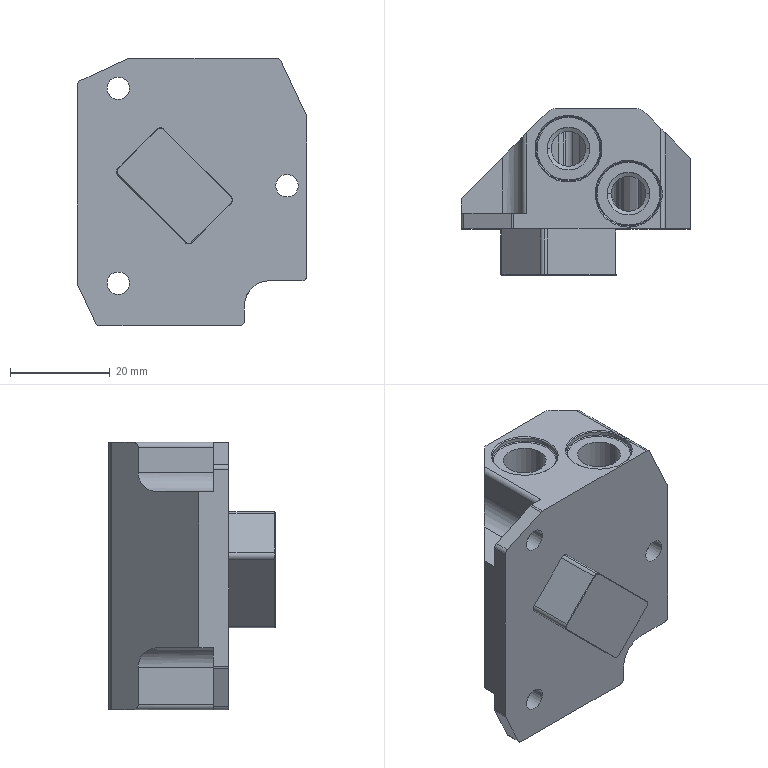NC program | NX | posted with a generic post | part box 46 x 33.25 x 53.5 mm
Lines 2851 to 4234 of 9227:
(动态粗_COPY , TOOL : D5-15-D6-50-3T-ROUGH)
N5694 T03 M6
N5696 G53
N5698 G17 G0 G90 X31.076 Y-9.617 B0. C0. S5500 M3
N5700 G43 Z30.1 H3
N5702 Z-20.3
N5704 G94 G1 X31.051 Y-9.615 Z-20.456 F1500.
N5706 X31.026 Y-9.613 Z-20.518
N5708 X31.001 Y-9.611 Z-20.563
N5710 X30.976 Y-9.609 Z-20.6
N5712 X30.952 Y-9.607 Z-20.631
N5714 X30.927 Y-9.605 Z-20.657
N5716 X30.902 Y-9.603 Z-20.68
N5718 X30.877 Y-9.601 Z-20.7
N5720 X30.852 Y-9.598 Z-20.718
N5722 X30.827 Y-9.596 Z-20.733
N5724 X30.802 Y-9.594 Z-20.747
N5726 X30.777 Y-9.592 Z-20.758
N5728 X30.752 Y-9.59 Z-20.768
N5730 X30.727 Y-9.588 Z-20.777
N5732 X30.702 Y-9.586 Z-20.784
N5734 X30.677 Y-9.584 Z-20.79
N5736 X30.653 Y-9.582 Z-20.794
N5738 X30.628 Y-9.58 Z-20.797
N5740 X30.603 Y-9.578 Z-20.799
N5742 X30.578 Y-9.576 Z-20.8
N5744 X29.881 Y-9.517
N5746 G3 X29.337 Y-9.964 R0.505
N5748 G2 X29.126 Y-11.124 R4.721
N5750 X27.743 Y-15.478 R16.822
N5752 X24.485 Y-22.499 R210.996
N5754 X21.62 Y-24.637 R4.462
N5756 X18.467 Y-25.056 R15.527
N5758 G3 X18.186 Y-25.222 R1.339
N5760 G2 X16.95 Y-25.594 R2.967
N5762 G3 X18.297 Y-25.133 R2.665
N5764 G2 X19.134 Y-24.843 R2.024
N5766 G3 X21.771 Y-24.179 R14.32
N5768 X24.24 Y-21.945 R5.463
N5770 X26.382 Y-17.754 R38.745
N5772 X28.296 Y-13.146 R39.925
N5774 G1 X28.614 Y-12.016
N5776 G3 X29.204 Y-10.81 R3.559
N5778 G2 X28.449 Y-12.237 R3.854
N5780 G3 X27.157 Y-14.833 R19.594
N5782 G2 X24.386 Y-20.629 R79.826
N5784 X20.582 Y-23.809 R6.364
N5786 G3 X19.11 Y-24.321 R69.681
N5788 X18.705 Y-24.807 R2.122
N5790 G1 X18.353 Y-25.088
N5792 G3 X19.059 Y-24.335 R2.54
N5794 G2 X20.592 Y-23.523 R7.508
N5796 G3 X24.162 Y-20.237 R7.733
N5798 X26.636 Y-15.252 R50.491
N5800 G2 X27.833 Y-12.792 R25.129
N5802 G3 X28.551 Y-12.108 R10.707
N5804 G2 X27.648 Y-12.906 R4.578
N5806 G3 X26.327 Y-14.911 R7.951
N5808 G2 X24.13 Y-19.226 R117.584
N5810 X20.404 Y-22.922 R9.092
N5812 G3 X19.4 Y-23.594 R5.764
N5814 X19.102 Y-24.274 R6.577
N5816 G1 X19.035 Y-24.365
N5818 G3 X19.364 Y-23.624 R3.443
N5820 G2 X20.274 Y-22.765 R3.601
N5822 G3 X24.264 Y-18.269 R12.006
N5824 G2 X26.373 Y-14.245 R243.473
N5826 X27.133 Y-13.179 R5.241
N5828 G3 X27.788 Y-12.794 R14.693
N5830 G2 X26.949 Y-13.25 R5.193
N5832 G3 X25.575 Y-14.893 R5.368
N5834 G2 X23.525 Y-18.492 R562.436
N5836 X20.399 Y-21.972 R13.716
N5838 G3 X19.459 Y-22.946 R4.049
N5840 G1 X19.351 Y-23.659
N5842 G2 X19.511 Y-22.778 R3.04
N5844 X20.59 Y-21.491 R5.992
N5846 G3 X24.171 Y-16.732 R18.8
N5848 G2 X25.976 Y-13.884 R19.759
N5850 X26.532 Y-13.366 R2.468
N5852 G1 X27.117 Y-13.162
N5854 G3 X26.179 Y-13.499 R7.877
N5856 X24.693 Y-15.069 R5.396
N5858 G2 X22.527 Y-18.401 R233.076
N5860 X20.094 Y-21.278 R33.455
N5862 G3 X19.445 Y-22.239 R3.013
N5864 G1 X19.435 Y-23.001
N5866 G2 X19.459 Y-22.097 R5.398
N5868 X20.46 Y-20.515 R5.211
N5870 G3 X23.859 Y-15.792 R39.523
N5872 G2 X25.574 Y-13.698 R9.325
N5874 X26.057 Y-13.415 R1.415
N5876 G1 X26.542 Y-13.361
N5878 G3 X25.521 Y-13.563 R2.86
N5880 X23.893 Y-15.066 R5.4
N5882 G1 X21.463 Y-18.418
N5884 G3 X19.635 Y-20.87 R32.6
N5886 X19.435 Y-21.333 R1.332
N5888 G1 Y-22.271
N5890 G2 X19.454 Y-21.126 R24.422
N5892 X20.404 Y-19.386 R5.786
N5894 X23.602 Y-14.996 R166.387
N5896 X25.321 Y-13.478 R5.337
N5898 X25.898 Y-13.433 R9.861
N5900 G3 X25.111 Y-13.481 R7.526
N5902 X23.474 Y-14.611 R3.969
N5904 X20.694 Y-18.143 R37.147
N5906 X19.449 Y-20.142 R10.513
N5908 G1 X19.435 Y-21.274
N5910 G2 X19.454 Y-20.01 R39.949
N5912 X20.44 Y-18.073 R6.448
N5914 X23.284 Y-14.448 R25.188
N5916 X24.707 Y-13.46 R4.137
N5918 G1 X25.306 Y-13.45
N5920 G3 X24.216 Y-13.532 R3.271
N5922 X22.355 Y-14.893 R5.19
N5924 X19.521 Y-18.773 R18.084
N5926 G1 X19.436 Y-19.04
N5928 X19.435 Y-20.165
N5930 X19.452 Y-18.824
N5932 G2 X20.487 Y-16.784 R6.292
N5934 X23.122 Y-13.899 R11.922
N5936 X24.011 Y-13.45 R2.38
N5938 G1 X24.611
N5940 G3 X23.467 Y-13.516 R4.027
N5942 X21.53 Y-14.857 R5.115
N5944 X19.45 Y-17.764 R10.096
N5946 G1 X19.436 Y-18.981
N5948 X19.451 Y-17.645
N5950 G2 X20.552 Y-15.608 R5.519
N5952 X22.87 Y-13.561 R7.086
N5954 X23.202 Y-13.45 R2.139
N5956 G1 X23.802
N5958 G3 X22.657 Y-13.512 R4.284
N5960 X20.539 Y-15.037 R5.056
N5962 X19.447 Y-16.671 R5.979
N5964 G1 X19.436 Y-17.797
N5966 G2 X19.455 Y-16.534 R20.679
N5968 X20.843 Y-14.421 R4.737
N5970 X22.332 Y-13.455 R4.05
N5972 G1 X23.012 Y-13.45
N5974 G3 X21.84 Y-13.511 R4.409
N5976 X19.452 Y-15.697 R4.316
N5978 G1 X19.436 Y-16.702
N5980 G2 X19.457 Y-15.587 R9.901
N5982 X21.553 Y-13.454 R3.485
N5984 G1 X22.153 Y-13.45
N5986 G3 X21.094 Y-13.509 R3.922
N5988 X19.451 Y-14.943 R2.775
N5990 G1 X19.436 Y-15.753
N5992 G2 X19.462 Y-14.824 R4.155
N5994 X20.895 Y-13.452 R2.243
N5996 G1 X21.405 Y-13.45
N5998 G3 X20.386 Y-13.539 R2.784
N6000 X19.516 Y-14.351 R1.427
N6002 X19.436 Y-14.992 R2.942
N6004 G2 X19.926 Y-13.753 R1.462
N6006 X20.573 Y-13.481 R1.202
N6008 X21.173 Y-13.945 R0.505
N6010 G1 X21.192 Y-14.367
N6012 G2 X21.037 Y-14.678 R0.515
N6014 G1 X21.019 Y-14.695 Z-20.799
N6016 X21.001 Y-14.712 Z-20.797
N6018 X20.983 Y-14.73 Z-20.794
N6020 X20.964 Y-14.747 Z-20.79
N6022 X20.946 Y-14.764 Z-20.784
N6024 X20.928 Y-14.781 Z-20.777
N6026 X20.91 Y-14.798 Z-20.768
N6028 X20.892 Y-14.816 Z-20.758
N6030 X20.873 Y-14.833 Z-20.747
N6032 X20.855 Y-14.85 Z-20.733
N6034 X20.837 Y-14.867 Z-20.718
N6036 X20.819 Y-14.884 Z-20.7
N6038 X20.801 Y-14.901 Z-20.68
N6040 X20.783 Y-14.919 Z-20.657
N6042 X20.764 Y-14.936 Z-20.631
N6044 X20.746 Y-14.953 Z-20.6
N6046 X20.728 Y-14.97 Z-20.563
N6048 X20.71 Y-14.987 Z-20.518
N6050 X20.692 Y-15.004 Z-20.456
N6052 X20.674 Y-15.022 Z-20.3
N6054 G0 Z30.1
N6056 X-12.085 Y-26.828
N6058 Z-20.3
N6060 G1 X-12.11 Z-20.456
N6062 X-12.135 Z-20.518
N6064 X-12.16 Z-20.563
N6066 X-12.185 Z-20.6
N6068 X-12.21 Z-20.631
N6070 X-12.235 Z-20.657
N6072 X-12.26 Z-20.68
N6074 X-12.285 Z-20.7
N6076 X-12.31 Z-20.718
N6078 X-12.335 Z-20.733
N6080 X-12.36 Z-20.747
N6082 X-12.385 Z-20.758
N6084 X-12.41 Z-20.768
N6086 X-12.435 Z-20.777
N6088 X-12.46 Z-20.784
N6090 X-12.485 Z-20.79
N6092 X-12.51 Z-20.794
N6094 X-12.535 Z-20.797
N6096 X-12.56 Z-20.799
N6098 X-12.585 Z-20.8
N6100 G2 X-13.047 Y-26.527 R0.506
N6102 G1 X-13.202 Y-26.168
N6104 X-13.373 Y-25.816
N6106 G3 X-13.787 Y-25.6 R0.508
N6108 G2 X-15.607 Y-25.397 R7.506
N6110 X-17.835 Y-25.157 R69.571
N6112 X-21.479 Y-23.892 R17.184
N6114 X-26.417 Y-21.578 R103.757
N6116 X-28.452 Y-18.791 R4.417
N6118 X-28.893 Y-15.038 R16.18
N6120 G1 X-28.954 Y-11.525
N6122 X-29.26 Y-10.651
N6124 G2 X-29.35 Y-9.437 R7.155
N6126 G3 X-28.917 Y-11.57 R4.292
N6128 G2 X-28.642 Y-14.012 R11.018
N6130 G3 X-28.304 Y-17.814 R25.107
N6132 X-25.963 Y-21.251 R5.114
N6134 X-21.906 Y-23.363 R29.004
N6136 X-18.168 Y-24.708 R18.402
N6138 G1 X-15.887 Y-25.08
N6140 G3 X-15.009 Y-25.511 R3.058
N6142 G2 X-16.006 Y-24.976 R2.885
N6144 G3 X-17.82 Y-24.332 R9.627
N6146 G2 X-24.99 Y-21.198 R32.607
N6148 X-27.623 Y-17.462 R5.932
N6150 X-28.125 Y-13.845 R21.529
N6152 G3 X-28.335 Y-12.362 R7.06
N6154 G2 X-28.984 Y-11.428 R6.039
N6156 G3 X-28.335 Y-12.327 R3.58
N6158 G2 X-27.887 Y-13.954 R4.664
N6160 G3 X-27.299 Y-17.276 R24.892
N6162 X-24.464 Y-21.028 R6.502
N6164 X-18.113 Y-23.906 R26.819
N6166 G2 X-16.446 Y-24.518 R11.795
N6168 G1 X-16.174 Y-24.838
N6170 X-15.936 Y-25.021
N6172 G2 X-16.504 Y-24.42 R2.303
N6174 G3 X-18.187 Y-23.466 R5.904
N6176 G2 X-22.785 Y-21.386 R52.481
N6178 X-25.637 Y-19.034 R8.191
N6180 X-27.048 Y-15.506 R9.268
N6182 G3 X-27.651 Y-12.973 R18.748
N6184 X-27.995 Y-12.665 R0.838
N6186 G1 X-28.366 Y-12.293
N6188 G3 X-27.725 Y-12.837 R2.213
N6190 G2 X-27.098 Y-14.225 R3.503
N6192 G3 X-26.135 Y-17.336 R22.654
N6194 X-22.893 Y-20.88 R7.855
N6196 X-18.602 Y-22.962 R33.207
N6198 G2 X-16.774 Y-23.949 R8.305
N6200 X-16.587 Y-24.3 R1.523
N6202 G1 X-16.45 Y-24.479
N6204 G2 X-16.774 Y-23.879 R2.246
N6206 G3 X-18.238 Y-22.732 R4.268
N6208 G2 X-21.662 Y-20.972 R473.58
N6210 X-24.938 Y-18.088 R8.981
N6212 X-26.19 Y-15.326 R12.038
N6214 G3 X-27. Y-13.299 R10.69
N6216 X-27.312 Y-13.093 R0.723
N6218 G1 X-27.757 Y-12.814
N6220 G3 X-27.035 Y-13.222 R7.421
N6222 G2 X-26.21 Y-14.598 R3.981
N6224 G3 X-24.829 Y-17.552 R19.21
N6226 X-21.397 Y-20.704 R9.675
N6228 G1 X-18.113 Y-22.49
N6230 G2 X-16.921 Y-23.437 R4.496
N6232 G1 X-16.863 Y-23.575
N6234 G2 X-16.99 Y-24.042 R0.502
N6236 G1 X-17.379 Y-24.342 Z-20.75
N6238 X-17.775 Y-24.633 Z-20.7
N6240 X-18.116 Y-24.878 F15000.
N6242 G2 X-18.777 Y-24.68 R0.5
N6244 G1 X-18.865 Y-24.527
N6246 X-18.925 Y-24.362
N6248 G2 X-18.055 Y-23.947 R0.5
N6250 G1 X-17.781 Y-24.247 Z-20.741 F1500.
N6252 X-17.498 Y-24.538 Z-20.783
N6254 X-17.349 Y-24.617 Z-20.8
N6256 G3 X-16.732 Y-23.95 R0.5
N6258 G2 X-16.924 Y-23.331 R3.912
N6260 G3 X-18.193 Y-22.05 R3.71
N6262 X-21.234 Y-20.187 R165.735
N6264 G2 X-25.128 Y-15.659 R10.283
N6266 G3 X-26.236 Y-13.621 R13.141
N6268 X-26.553 Y-13.359 R0.755
N6270 G1 X-27.154 Y-13.149
N6272 G2 X-26.305 Y-13.479 R4.099
N6274 X-25.199 Y-14.979 R5.065
N6276 G3 X-23.192 Y-18.028 R15.991
N6278 X-20.093 Y-20.498 R13.845
N6280 G2 X-17.562 Y-22.236 R18.05
N6282 X-16.928 Y-23.058 R2.046
N6284 G1 X-16.869 Y-23.504
N6286 G3 X-17.094 Y-22.518 R2.548
N6288 X-18.645 Y-20.954 R5.492
N6290 G2 X-21.491 Y-18.859 R49.445
N6292 X-24.182 Y-15.62 R13.293
N6294 G3 X-25.592 Y-13.661 R10.79
N6296 X-25.975 Y-13.425 R0.85
N6298 G1 X-26.551 Y-13.36
N6300 G2 X-25.771 Y-13.475 R3.56
N6302 X-24.563 Y-14.634 R3.768
N6304 G3 X-22.429 Y-17.445 R33.621
N6306 X-19.235 Y-20.148 R20.206
N6308 G2 X-17.235 Y-21.954 R9.286
N6310 X-16.936 Y-22.974 R1.272
N6312 G3 X-17.496 Y-21.247 R2.183
N6314 X-19.239 Y-19.599 R12.076
N6316 G2 X-23.501 Y-15.2 R20.861
N6318 G3 X-25.085 Y-13.525 R7.47
N6320 X-25.751 Y-13.45 R1.357
N6322 G1 X-25.937 Y-13.429
N6324 X-25.22 Y-13.452
N6326 G2 X-24.01 Y-14.274 R2.795
N6328 X-21.862 Y-16.738 R121.025
N6330 G3 X-18.752 Y-19.617 R34.105
N6332 G2 X-17.072 Y-21.512 R7.478
N6334 X-16.936 Y-21.884 R1.731
N6336 G1 Y-22.446
N6338 G3 X-16.995 Y-21.391 R3.87
N6340 X-18.224 Y-19.591 R4.969
N6342 G2 X-21.057 Y-16.815 R194.434
N6344 G3 X-23.468 Y-14.185 R85.675
N6346 X-24.45 Y-13.467 R3.465
N6348 G1 X-25.27 Y-13.45
N6350 G2 X-24.35 Y-13.472 R7.141
N6352 X-22.799 Y-14.553 R4.233
N6354 G3 X-18.255 Y-19.159 R172.662
N6356 G2 X-16.946 Y-21.035 R5.661
N6358 G1 X-16.936 Y-21.71
N6360 G3 X-17. Y-20.559 R4.188
N6362 X-18.242 Y-18.615 R5.756
N6364 X-22.362 Y-14.335 R107.426
N6366 X-23.569 Y-13.47 R5.09
N6368 X-24.504 Y-13.45 R10.48
N6370 G2 X-23.47 Y-13.472 R9.077
N6372 X-21.855 Y-14.507 R4.566
N6374 X-17.78 Y-18.755 R46.322
N6376 X-16.941 Y-20.2 R4.92
N6378 G1 X-16.936 Y-20.919
N6380 G3 X-16.992 Y-19.696 R5.168
N6382 X-18.23 Y-17.611 R6.185
N6384 X-21.842 Y-13.955 R25.45
N6386 X-22.703 Y-13.454 R2.671
N6388 G1 X-23.64 Y-13.45
N6390 G2 X-22.524 Y-13.473 R8.444
N6392 X-20.766 Y-14.572 R4.957
N6394 X-17.418 Y-18.291 R19.641
N6396 X-16.936 Y-19.321 R3.21
N6398 G1 Y-20.033
N6400 G3 X-16.984 Y-18.765 R6.188
N6402 X-18.238 Y-16.564 R6.312
N6404 X-21.282 Y-13.665 R13.419
N6406 X-21.775 Y-13.45 R1.294
N6408 G1 X-22.675
N6410 G2 X-21.558 Y-13.47 R11.954
N6412 X-19.785 Y-14.563 R4.796
N6414 X-17.095 Y-17.881 R11.319
N6416 X-16.936 Y-18.338 R2.62
N6418 G1 Y-19.088
N6420 G3 X-16.988 Y-17.753 R6.433
N6422 X-18.307 Y-15.48 R6.168
N6424 X-20.661 Y-13.479 R7.824
N6426 X-21.707 Y-13.45 R5.938
N6428 G2 X-20.595 Y-13.469 R17.143
N6430 X-18.774 Y-14.647 R4.564
N6432 X-16.949 Y-17.249 R7.142
N6434 G1 X-16.936 Y-18.083
N6436 G3 X-16.983 Y-16.772 R6.605
N6438 X-18.644 Y-14.26 R5.568
N6440 X-19.808 Y-13.46 R3.617
N6442 G1 X-20.745 Y-13.45
N6444 G2 X-19.669 Y-13.471 R9.363
N6446 X-17.898 Y-14.744 R4.011
N6448 X-16.939 Y-16.341 R4.52
N6450 G1 X-16.936 Y-17.091
N6452 G3 X-16.987 Y-15.823 R5.741
N6454 X-18.918 Y-13.477 R4.112
N6456 X-19.808 Y-13.45 R4.003
N6458 G2 X-18.844 Y-13.474 R5.75
N6460 X-16.937 Y-15.499 R3.221
N6462 G1 X-16.936 Y-16.149
N6464 G3 X-16.975 Y-15.061 R4.878
N6466 X-18.259 Y-13.472 R2.592
N6468 X-19.013 Y-13.45 R5.62
N6470 G2 X-18.153 Y-13.48 R3.964
N6472 X-16.939 Y-14.792 R2.113
N6474 G1 X-16.936 Y-15.316
N6476 G3 X-17.11 Y-14.14 R2.379
N6478 X-18.188 Y-13.46 R1.281
N6480 G1 X-18.325 Y-13.45
N6482 G2 X-17.304 Y-13.848 R1.499
N6484 X-16.99 Y-14.457 R1.399
N6486 X-17.54 Y-15.05 R0.505
N6488 G1 X-18.164 Y-14.984
N6490 X-18.189 Y-14.981 Z-20.799
N6492 X-18.213 Y-14.979 Z-20.797
N6494 X-18.238 Y-14.976 Z-20.794
N6496 X-18.263 Y-14.973 Z-20.79
N6498 X-18.288 Y-14.971 Z-20.784
N6500 X-18.313 Y-14.968 Z-20.777
N6502 X-18.338 Y-14.965 Z-20.768
N6504 X-18.363 Y-14.963 Z-20.758
N6506 X-18.387 Y-14.96 Z-20.747
N6508 X-18.412 Y-14.957 Z-20.733
N6510 X-18.437 Y-14.955 Z-20.718
N6512 X-18.462 Y-14.952 Z-20.7
N6514 X-18.487 Y-14.949 Z-20.68
N6516 X-18.512 Y-14.947 Z-20.657
N6518 X-18.537 Y-14.944 Z-20.631
N6520 X-18.561 Y-14.942 Z-20.6
N6522 X-18.586 Y-14.939 Z-20.563
N6524 X-18.611 Y-14.936 Z-20.518
N6526 X-18.636 Y-14.934 Z-20.456
N6528 X-18.661 Y-14.931 Z-20.3
N6530 G0 Z30.1
N6532 X-24.518 Y14.833
N6534 Z-6.433
N6536 G1 X-24.519 Y14.808 Z-6.589
N6538 X-24.52 Y14.784 Z-6.651
N6540 X-24.521 Y14.759 Z-6.697
N6542 X-24.522 Y14.734 Z-6.733
N6544 X-24.523 Y14.709 Z-6.764
N6546 X-24.524 Y14.684 Z-6.79
N6548 X-24.525 Y14.659 Z-6.813
N6550 X-24.526 Y14.634 Z-6.833
N6552 X-24.527 Y14.609 Z-6.851
N6554 X-24.528 Y14.584 Z-6.866
N6556 X-24.529 Y14.559 Z-6.88
N6558 X-24.53 Y14.534 Z-6.892
N6560 X-24.531 Y14.509 Z-6.902
N6562 X-24.532 Y14.484 Z-6.91
N6564 X-24.533 Y14.459 Z-6.917
N6566 X-24.534 Y14.434 Z-6.923
N6568 X-24.535 Y14.409 Z-6.928
N6570 X-24.536 Y14.384 Z-6.931
N6572 X-24.537 Y14.359 Z-6.933
N6574 X-24.538 Y14.334
N6576 X-24.567 Y13.635
N6578 G3 X-24.059 Y13.109 R0.505
N6580 X-22.612 Y13.242 R4.347
N6582 X-20.35 Y15.655 R3.586
N6584 G1 Y17.043
N6586 G2 X-20.38 Y15.307 R14.49
N6588 X-22.485 Y13.123 R3.25
N6590 G1 X-23.235 Y13.115
N6592 G3 X-21.88 Y13.269 R3.479
N6594 X-20.362 Y15.398 R2.372
N6596 X-20.975 Y15.947 R0.505
N6598 G1 X-21.581 Y15.81
N6600 X-21.605 Y15.804
N6602 X-21.629 Y15.799 Z-6.931
N6604 X-21.654 Y15.793 Z-6.928
N6606 X-21.678 Y15.788 Z-6.923
N6608 X-21.703 Y15.782 Z-6.917
N6610 X-21.727 Y15.777 Z-6.91
N6612 X-21.751 Y15.771 Z-6.902
N6614 X-21.776 Y15.766 Z-6.892
N6616 X-21.8 Y15.76 Z-6.88
N6618 X-21.825 Y15.755 Z-6.866
N6620 X-21.849 Y15.749 Z-6.851
N6622 X-21.873 Y15.744 Z-6.833
N6624 X-21.898 Y15.738 Z-6.813
N6626 X-21.922 Y15.733 Z-6.79
N6628 X-21.946 Y15.727 Z-6.764
N6630 X-21.971 Y15.722 Z-6.733
N6632 X-21.995 Y15.716 Z-6.697
N6634 X-22.02 Y15.71 Z-6.651
N6636 X-22.044 Y15.705 Z-6.589
N6638 X-22.068 Y15.699 Z-6.433
N6640 G0 Z30.1
N6642 X-24.57 Y14.824
N6644 Z-13.367
N6646 G1 X-24.571 Y14.799 Z-13.523
N6648 X-24.573 Y14.774 Z-13.585
N6650 X-24.574 Y14.749 Z-13.63
N6652 X-24.575 Y14.724 Z-13.667
N6654 X-24.576 Y14.699 Z-13.697
N6656 X-24.577 Y14.674 Z-13.724
N6658 X-24.578 Y14.649 Z-13.747
N6660 X-24.579 Y14.624 Z-13.767
N6662 X-24.58 Y14.599 Z-13.784
N6664 X-24.582 Y14.574 Z-13.8
N6666 X-24.583 Y14.549 Z-13.813
N6668 X-24.584 Y14.524 Z-13.825
N6670 X-24.585 Y14.5 Z-13.835
N6672 X-24.586 Y14.475 Z-13.844
N6674 X-24.587 Y14.45 Z-13.851
N6676 X-24.588 Y14.425 Z-13.857
N6678 X-24.589 Y14.4 Z-13.861
N6680 X-24.59 Y14.375 Z-13.864
N6682 X-24.592 Y14.35 Z-13.866
N6684 X-24.593 Y14.325 Z-13.867
N6686 X-24.624 Y13.628
N6688 G3 X-24.119 Y13.1 R0.505
N6690 X-22.613 Y13.247 R4.23
N6692 X-20.35 Y15.689 R3.585
N6694 G1 Y17.039
N6696 G2 X-20.371 Y15.394 R23.318
N6698 X-22.518 Y13.115 R3.248
N6700 G1 X-23.367 Y13.1
N6702 G3 X-21.88 Y13.269 R3.867
N6704 X-20.35 Y15.606 R2.439
N6706 X-20.803 Y16.108 R0.505
N6708 G1 X-21.581 Y16.188
N6710 X-21.606 Y16.19 Z-13.866
N6712 X-21.631 Y16.193 Z-13.864
N6714 X-21.655 Y16.195 Z-13.861
N6716 X-21.68 Y16.198 Z-13.857
N6718 X-21.705 Y16.201 Z-13.851
N6720 X-21.73 Y16.203 Z-13.844
N6722 X-21.755 Y16.206 Z-13.835
N6724 X-21.78 Y16.208 Z-13.825
N6726 X-21.805 Y16.211 Z-13.813
N6728 X-21.83 Y16.213 Z-13.8
N6730 X-21.854 Y16.216 Z-13.784
N6732 X-21.879 Y16.218 Z-13.767
N6734 X-21.904 Y16.221 Z-13.747
N6736 X-21.929 Y16.224 Z-13.724
N6738 X-21.954 Y16.226 Z-13.697
N6740 X-21.979 Y16.229 Z-13.667
N6742 X-22.004 Y16.231 Z-13.63
N6744 X-22.029 Y16.234 Z-13.585
N6746 X-22.053 Y16.236 Z-13.523
N6748 X-22.078 Y16.239 Z-13.367
N6750 G0 Z30.1
N6752 X-24.53 Y14.832
N6754 Z-20.3
N6756 G1 X-24.532 Y14.807 Z-20.456
N6758 X-24.533 Y14.782 Z-20.518
N6760 X-24.534 Y14.757 Z-20.563
N6762 X-24.535 Y14.732 Z-20.6
N6764 X-24.536 Y14.707 Z-20.631
N6766 X-24.538 Y14.682 Z-20.657
N6768 X-24.539 Y14.657 Z-20.68
N6770 X-24.54 Y14.632 Z-20.7
N6772 X-24.541 Y14.607 Z-20.718
N6774 X-24.543 Y14.582 Z-20.733
N6776 X-24.544 Y14.557 Z-20.747
N6778 X-24.545 Y14.532 Z-20.758
N6780 X-24.546 Y14.507 Z-20.768
N6782 X-24.547 Y14.482 Z-20.777
N6784 X-24.549 Y14.457 Z-20.784
N6786 X-24.55 Y14.432 Z-20.79
N6788 X-24.551 Y14.407 Z-20.794
N6790 X-24.552 Y14.382 Z-20.797
N6792 X-24.554 Y14.358 Z-20.799
N6794 X-24.555 Y14.333 Z-20.8
N6796 X-24.589 Y13.64
N6798 G3 X-24.081 Y13.11 R0.505
N6800 X-22.616 Y13.248 R4.366
N6802 X-20.35 Y15.667 R3.615
N6804 G1 Y17.054
N6806 G2 X-20.376 Y15.358 R16.596
N6808 X-22.535 Y13.119 R3.185
N6810 G1 X-23.322 Y13.115
N6812 G3 X-21.989 Y13.23 R4.057
N6814 X-20.35 Y15.568 R2.404
N6816 X-20.799 Y16.07 R0.505
N6818 G1 X-21.581 Y16.158
N6820 X-21.606 Y16.16 Z-20.799
N6822 X-21.631 Y16.163 Z-20.797
N6824 X-21.655 Y16.166 Z-20.794
N6826 X-21.68 Y16.169 Z-20.79
N6828 X-21.705 Y16.171 Z-20.784
N6830 X-21.73 Y16.174 Z-20.777
N6832 X-21.755 Y16.177 Z-20.768
N6834 X-21.78 Y16.18 Z-20.758
N6836 X-21.804 Y16.183 Z-20.747
N6838 X-21.829 Y16.185 Z-20.733
N6840 X-21.854 Y16.188 Z-20.718
N6842 X-21.879 Y16.191 Z-20.7
N6844 X-21.904 Y16.194 Z-20.68
N6846 X-21.929 Y16.196 Z-20.657
N6848 X-21.954 Y16.199 Z-20.631
N6850 X-21.978 Y16.202 Z-20.6
N6852 X-22.003 Y16.205 Z-20.563
N6854 X-22.028 Y16.208 Z-20.518
N6856 X-22.053 Y16.21 Z-20.456
N6858 X-22.078 Y16.213 Z-20.3
N6860 G0 Z30.1
N6862 X-22.07 Y19.402
N6864 Z-6.433
N6866 G1 X-22.045 Y19.397 Z-6.589
N6868 X-22.021 Y19.393 Z-6.651
N6870 X-21.996 Y19.388 Z-6.697
N6872 X-21.972 Y19.383 Z-6.733
N6874 X-21.947 Y19.378 Z-6.764
N6876 X-21.923 Y19.373 Z-6.79
N6878 X-21.898 Y19.368 Z-6.813
N6880 X-21.874 Y19.363 Z-6.833
N6882 X-21.849 Y19.359 Z-6.851
N6884 X-21.825 Y19.354 Z-6.866
N6886 X-21.8 Y19.349 Z-6.88
N6888 X-21.776 Y19.344 Z-6.892
N6890 X-21.751 Y19.339 Z-6.902
N6892 X-21.727 Y19.334 Z-6.91
N6894 X-21.702 Y19.329 Z-6.917
N6896 X-21.678 Y19.325 Z-6.923
N6898 X-21.653 Y19.32 Z-6.928
N6900 X-21.628 Y19.315 Z-6.931
N6902 X-21.604 Y19.31 Z-6.933
N6904 X-21.579 Y19.305
N6906 X-21.223 Y19.231
N6908 X-20.863 Y19.173
N6910 G3 X-20.359 Y19.683 R0.505
N6912 G2 X-20.008 Y21.245 R3.266
N6914 X-18.427 Y22.479 R2.827
N6916 G1 X-17.749 Y22.575
N6918 X-2.649
N6920 G2 X-0.803 Y21.793 R2.82
N6922 G3 X0.746 Y21.074 R3.932
N6924 X3.114 Y21.564 R4.522
N6926 G2 X4.473 Y22.479 R2.867
N6928 G1 X5.151 Y22.575
N6930 X21.476
N6932 G2 X22.391 Y22.403 R3.105
N6934 G3 X23.017 Y23.074 R0.5
N6936 X22.74 Y23.362 Z-6.892 R0.728
N6938 G1 X22.276 Y23.705 Z-6.833
N6940 X21.899 Y23.988 F15000.
N6942 X21.516 Y24.261
N6944 X21.404 Y24.301
N6946 X21.286 Y24.317
N6948 X9.168
N6950 G3 X5.176 Y24.081 R34.003
N6952 G1 X3.187 Y23.844
N6954 G3 X2.791 Y23.141 R0.5
N6956 G1 X2.846 Y23.019
N6958 X3.251 Y22.124 Z-6.933 F1500.
N6960 G2 X3.187 Y21.634 R0.502
N6962 X2.065 Y21.019 R2.104
N6964 X-0.508 Y21.409 R3.053
N6966 G1 X-0.803 Y21.793
N6968 G3 X0.02 Y20.942 R2.619
N6970 X2.717 Y20.979 R2.924
N6972 G1 X2.856 Y21.154
N6974 G3 X2.806 Y21.669 R0.552
N6976 X2.317 Y21.922 Z-6.875 R0.596
N6978 G1 X1.91 Y21.966 Z-6.833
N6980 X0.497 Y22.119 F15000.
N6982 X-0.003 Y22.168 Z-6.885 F1500.
N6984 G3 X-0.416 Y21.956 Z-6.933 R0.559
N6986 X-0.421 Y21.287 R0.551
N6988 X0.816 Y20.443 R1.68
N6990 X2.564 Y20.639 R2.514
N6992 X2.893 Y21.245 R1.388
N6994 G1 X3.164 Y21.604
N6996 G3 X2.684 Y20.737 R2.228
N6998 G2 X1.628 Y20.256 R1.48
N7000 X-0.18 Y20.788 R2.26
N7002 X-0.373 Y21.204 R5.722
N7004 G3 X0.123 Y20.403 R1.562
N7006 X2.47 Y20.302 R2.112
N7008 X2.624 Y20.555 R1.204
N7010 X2.518 Y21.033 R0.553
N7012 X2.079 Y21.246 Z-6.882 R0.615
N7014 G1 X1.604 Y21.318 Z-6.833
N7016 X0.865 Y21.431 F15000.
N7018 X0.317 Y21.508 Z-6.89 F1500.
N7020 G3 X-0.069 Y21.348 Z-6.933 R0.566
N7022 X-0.19 Y20.752 R0.551
N7024 X0.93 Y19.842 R1.458
N7026 X2.446 Y20.075 R1.763
N7028 X2.635 Y20.612 R0.767
N7030 G1 X2.706 Y20.785
N7032 G3 X2.577 Y20.22 R1.964
N7034 G2 X1.677 Y19.682 R1.129
N7036 X-0.057 Y20.312 R1.826
N7038 G1 X-0.112 Y20.451
N7040 G2 X0.063 Y20.978 R0.552
N7042 X0.588 Y21.099 Z-6.876 R0.601
N7044 G1 X1.007 Y21.046 Z-6.833
N7046 X1.463 Y20.989 F15000.
N7048 X2.197 Y20.891 Z-6.909 F1500.
N7050 X2.308 Y20.844 Z-6.921
N7052 X2.408 Y20.778 Z-6.933
N7054 G2 X2.595 Y20.292 R0.552
N7056 X1.983 Y19.665 R0.849
N7058 X-0.013 Y20.106 R1.823
N7060 X-0.134 Y20.612 R1.134
N7062 G3 X0.005 Y19.978 R1.387
N7064 X2.433 Y19.724 R1.709
N7066 X2.593 Y20.274 R0.907
N7068 G2 X2.438 Y19.683 R1.097
N7070 X0.596 Y19.374 R1.629
N7072 X-0.059 Y20.005 R1.006
N7074 G1 X-0.087 Y20.229
N7076 G3 X0.695 Y19.154 R1.087
N7078 X2.457 Y19.474 R1.575
N7080 X2.55 Y19.934 R0.768
N7082 G2 X2.062 Y19.091 R0.771
N7084 X0.003 Y19.572 R1.621
N7086 X-0.05 Y19.932 R1.053
N7088 G3 X0.483 Y18.956 R0.933
N7090 X2.445 Y19.161 R1.611
N7092 X2.55 Y19.708 R0.807
N7094 G2 X2.044 Y18.782 R0.827
N7096 X0.003 Y19.283 R1.598
N7098 X-0.05 Y19.67 R1.07
N7100 G3 X0.573 Y18.605 R1.
N7102 X2.459 Y18.883 R1.572
N7104 X2.55 Y19.414 R0.858
N7106 G2 X2.389 Y18.739 R0.848
N7108 X-0.009 Y19.016 R1.562
N7110 X-0.05 Y19.38 R1.439
N7112 G3 X0.565 Y18.308 R1.006
N7114 X2.399 Y18.521 R1.585
N7116 X2.55 Y19.091 R1.114
N7118 G2 X2.283 Y18.352 R1.
N7120 X0.009 Y18.69 R1.551
N7122 X-0.05 Y19.089 R2.062
N7124 G3 X1.006 Y17.858 R1.208
N7126 X2.162 Y18.088 R1.303
N7128 X2.479 Y18.643 R1.329
N7130 G2 X0.033 Y18.595 R1.283
N7132 G3 X1.898 Y17.899 R1.257
N7134 X2.073 Y18.537 R0.505
N7136 G1 X1.332 Y20.084
N7138 X1.321 Y20.107
N7140 X1.31 Y20.129 Z-6.931
N7142 X1.299 Y20.152 Z-6.928
N7144 X1.288 Y20.174 Z-6.923
N7146 X1.278 Y20.197 Z-6.917
N7148 X1.267 Y20.219 Z-6.91
N7150 X1.256 Y20.242 Z-6.902
N7152 X1.245 Y20.265 Z-6.892
N7154 X1.234 Y20.287 Z-6.88
N7156 X1.224 Y20.31 Z-6.866
N7158 X1.213 Y20.332 Z-6.851
N7160 X1.202 Y20.355 Z-6.833
N7162 X1.191 Y20.377 Z-6.813
N7164 X1.18 Y20.4 Z-6.79
N7166 X1.17 Y20.422 Z-6.764
N7168 X1.159 Y20.445 Z-6.733
N7170 X1.148 Y20.468 Z-6.697
N7172 X1.137 Y20.49 Z-6.651
N7174 X1.126 Y20.513 Z-6.589
N7176 X1.116 Y20.535 Z-6.433
N7178 G0 Z30.1
N7180 X-4.46 Y27.326
N7182 Z-20.3
N7184 G1 X-4.462 Y27.301 Z-20.456
N7186 X-4.465 Y27.276 Z-20.518
N7188 X-4.467 Y27.251 Z-20.563
N7190 X-4.469 Y27.226 Z-20.6
N7192 X-4.471 Y27.201 Z-20.631
N7194 X-4.473 Y27.177 Z-20.657
N7196 X-4.475 Y27.152 Z-20.68
N7198 X-4.478 Y27.127 Z-20.7
N7200 X-4.48 Y27.102 Z-20.718
N7202 X-4.482 Y27.077 Z-20.733
N7204 X-4.484 Y27.052 Z-20.747
N7206 X-4.486 Y27.027 Z-20.758
N7208 X-4.488 Y27.002 Z-20.768
N7210 X-4.49 Y26.977 Z-20.777
N7212 X-4.493 Y26.952 Z-20.784
N7214 X-4.495 Y26.927 Z-20.79
N7216 X-4.497 Y26.903 Z-20.794
N7218 X-4.499 Y26.878 Z-20.797
N7220 X-4.501 Y26.853 Z-20.799
N7222 X-4.503 Y26.828 Z-20.8
N7224 X-4.562 Y26.148
N7226 G3 X-4.059 Y25.6 R0.505
N7228 G2 X-2.135 Y25.382 R9.923
N7230 G3 X2.851 Y25.204 R46.891
N7232 X4.533 Y25.223 R15.445
N7234 G2 X6.563 Y25.6 R4.392
N7236 G3 X4.423 Y25.17 R4.372
N7238 G2 X1.912 Y24.94 R10.538
N7240 X-1.83 Y25.096 R24.511
N7242 G3 X-2.849 Y25.51 R4.419
N7244 G2 X-1.634 Y24.968 R4.02
N7246 G3 X0.651 Y24.534 R6.91
N7248 X3.641 Y24.62 R13.058
N7250 G1 X4.588 Y25.243
N7252 G3 X3.729 Y24.642 R3.817
N7254 G2 X2.006 Y24.279 R4.061
N7256 X-1.108 Y24.566 R9.462
N7258 X-1.405 Y24.815 R1.875
N7260 G1 X-1.723 Y25.014
N7262 G2 X-1.072 Y24.494 R2.658
N7264 G3 X0.842 Y23.925 R4.128
N7266 X3.13 Y24.074 R6.014
N7268 G1 X3.332 Y24.239
N7270 G3 X3.353 Y24.781 R0.552
N7272 X2.828 Y25.086 Z-20.735 R0.595
N7274 G1 X2.487 Y25.124 Z-20.7
N7276 X-0.282 Y25.434 F15000.
N7278 X-0.767 Y25.482 Z-20.75 F1500.
N7280 G3 X-1.189 Y25.258 Z-20.8 R0.559
N7282 X-1.135 Y24.544 R0.55
N7284 X0.554 Y23.655 R2.819
N7286 X2.869 Y23.692 R4.569
N7288 X3.102 Y23.874 R1.229
N7290 G2 X3.76 Y24.669 R2.846
N7292 G3 X3.04 Y23.78 R2.849
N7294 G2 X1.85 Y23.379 R1.974
N7296 X-0.592 Y23.896 R3.993
N7298 G1 X-0.835 Y24.245
N7300 G3 X0.53 Y23.204 R1.96
N7302 X2.683 Y23.286 R3.194
N7304 X2.883 Y23.505 R1.194
N7306 X2.854 Y24.027 R0.552
N7308 X2.382 Y24.296 Z-20.743 R0.599
N7310 G1 X1.969 Y24.363 Z-20.7
N7312 X0.388 Y24.619 F15000.
N7314 X-0.114 Y24.694 Z-20.752 F1500.
N7316 G3 X-0.535 Y24.509 Z-20.8 R0.56
N7318 X-0.589 Y23.852 R0.551
N7320 X0.806 Y22.88 R2.024
N7322 X2.606 Y23.011 R2.479
N7324 X2.907 Y23.562 R1.01
N7326 G1 X3.066 Y23.816
N7328 G3 X2.754 Y23.135 R2.211
N7330 G2 X1.798 Y22.668 R1.316
N7332 X-0.269 Y23.258 R2.598
N7334 G1 X-0.446 Y23.625
N7336 G3 X-0.207 Y23.104 R4.274
N7338 X2.502 Y22.663 R2.241
N7340 X2.79 Y23.23 R1.164
N7342 G2 X2.564 Y22.685 R1.866
N7344 X1.062 Y22.296 R1.767
N7346 X-0.173 Y22.919 R1.811
N7348 G1 X-0.302 Y23.263
N7350 G3 X0.892 Y22.112 R1.471
N7352 X2.498 Y22.4 R1.778
N7354 X2.653 Y22.836 R0.844
N7356 G2 X2.069 Y22.063 R0.803
N7358 X-0.048 Y22.519 R1.923
N7360 G1 X-0.124 Y22.689
N7362 G2 X0.035 Y23.198 R0.552
N7364 X0.556 Y23.34 Z-20.743 R0.601
N7366 G1 X0.976 Y23.303 Z-20.7
N7368 X1.49 Y23.258 F15000.
N7370 X1.848 Y23.228 Z-20.737 F1500.
N7372 X2.205 Y23.189 Z-20.773
N7374 X2.327 Y23.139 Z-20.787
N7376 X2.436 Y23.066 Z-20.8
N7378 G2 X2.617 Y22.594 R0.552
N7380 X2.031 Y21.956 R0.858
N7382 X-0.033 Y22.366 R1.826
N7384 X-0.165 Y22.872 R2.041
N7386 G1 X-0.078 Y22.352
N7388 G3 X1.31 Y21.603 R1.55
N7390 X2.506 Y22.077 R1.451
N7392 X2.614 Y22.566 R1.201
N7394 G2 X2.469 Y21.976 R1.037
N7396 X0.542 Y21.65 R1.663
N7398 X-0.081 Y22.27 R0.967
N7400 G1 X-0.106 Y22.494
N7402 G3 X0.622 Y21.438 R1.064
N7404 X2.438 Y21.703 R1.657
N7406 X2.575 Y22.224 R0.987
N7408 G2 X2.458 Y21.679 R1.124
N7410 X0.616 Y21.316 R1.582
N7412 X-0.039 Y21.923 R1.039
N7414 G1 X-0.071 Y22.186
N7416 G3 X0.697 Y21.105 R1.069
N7418 X2.458 Y21.438 R1.575
N7420 X2.55 Y21.972 R0.856
N7422 G2 X2.394 Y21.303 R0.851
N7424 X0.002 Y21.538 R1.579
N7426 X-0.05 Y21.92 R1.099
N7428 G3 X0.576 Y20.859 R0.996
N7430 X2.456 Y21.137 R1.581
N7432 X2.55 Y21.636 R0.808
N7434 G2 X1.983 Y20.71 R0.829
N7436 X0.007 Y21.236 R1.593
N7438 X-0.049 Y21.63 R1.035
N7440 G3 X0.579 Y20.558 R1.007
N7442 X2.456 Y20.836 R1.576
N7444 X2.55 Y21.374 R0.853
N7446 G2 X2.392 Y20.7 R0.856
N7448 X-0.009 Y20.975 R1.556
N7450 X-0.048 Y21.331 R1.561
N7452 G3 X0.582 Y20.256 R1.011
N7454 X2.456 Y20.535 R1.574
N7456 X2.55 Y21.073 R0.853
N7458 G2 X2.392 Y20.399 R0.856
N7460 X-0.007 Y20.674 R1.557
N7462 X-0.048 Y21.033 R1.513
N7464 G3 X0.595 Y19.949 R1.024
N7466 X2.456 Y20.234 R1.573
N7468 X2.55 Y20.772 R0.853
N7470 G2 X2.392 Y20.098 R0.856
N7472 X-0.01 Y20.378 R1.554
N7474 X-0.047 Y20.764 R1.645
N7476 G3 X0.596 Y19.647 R1.032
N7478 X2.456 Y19.933 R1.573
N7480 X2.55 Y20.471 R0.853
N7482 G2 X2.392 Y19.797 R0.856
N7484 X0.004 Y20.049 R1.57
N7486 X-0.046 Y20.463 R1.155
N7488 G3 X0.666 Y19.315 R1.063
N7490 X2.456 Y19.632 R1.564
N7492 X2.55 Y20.17 R0.853
N7494 G2 X2.392 Y19.496 R0.856
N7496 X0.002 Y19.758 R1.563
N7498 X-0.045 Y20.129 R1.198
N7500 G3 X0.598 Y19.047 R1.033
N7502 X2.456 Y19.332 R1.569
N7504 X2.55 Y19.87 R0.853
N7506 G2 X2.392 Y19.196 R0.855
N7508 X0.003 Y19.459 R1.563
N7510 X-0.045 Y19.83 R1.19
N7512 G3 X0.67 Y18.715 R1.055
N7514 X2.456 Y19.031 R1.559
N7516 X2.55 Y19.569 R0.853
N7518 G2 X2.392 Y18.896 R0.855
N7520 X0.004 Y19.159 R1.563
N7522 X-0.044 Y19.53 R1.186
N7524 G3 X0.671 Y18.415 R1.055
N7526 X2.454 Y18.732 R1.546
N7528 X2.55 Y19.24 R0.869
N7530 G2 X1.931 Y18.283 R0.873
N7532 X0.006 Y18.855 R1.576
N7534 X-0.043 Y19.266 R1.176
N7536 G3 X0.698 Y18.104 R1.072
N7538 X2.32 Y18.313 R1.562
N7540 X2.525 Y18.871 R1.042
N7542 G2 X1.452 Y17.879 R1.072
N7544 X0.073 Y18.476 R1.456
N7546 G1 X-0.033 Y18.864
N7548 G3 X2.322 Y18.308 R1.28
N7550 G2 X2.099 Y18.036 R0.834
N7552 X1.257 Y17.707 R1.371
N7554 X0.777 Y17.804 R1.538
N7556 G1 X0.57 Y17.91
N7558 G2 X0.386 Y18.475 R0.506
N7560 G1 X1.181 Y20.918
N7562 X1.187 Y20.939 Z-20.799
N7564 X1.194 Y20.961 Z-20.798
N7566 X1.201 Y20.982 Z-20.795
N7568 X1.208 Y21.004 Z-20.791
N7570 X1.215 Y21.025 Z-20.786
N7572 X1.222 Y21.047 Z-20.779
N7574 X1.229 Y21.068 Z-20.771
N7576 X1.236 Y21.09 Z-20.762
N7578 X1.243 Y21.111 Z-20.752
N7580 X1.25 Y21.133 Z-20.74
N7582 X1.257 Y21.154 Z-20.726
N7584 X1.264 Y21.175 Z-20.71
N7586 X1.271 Y21.197 Z-20.692
N7588 X1.278 Y21.218 Z-20.671
N7590 X1.285 Y21.24 Z-20.647
N7592 X1.292 Y21.261 Z-20.62
N7594 X1.299 Y21.283 Z-20.586
N7596 X1.306 Y21.304 Z-20.545
N7598 X1.313 Y21.326 Z-20.49
N7600 X1.32 Y21.347 Z-20.349
N7602 G0 Z30.1
N7604 X-1.193 Y26.715
N7606 Z-13.367
N7608 G1 X-1.203 Y26.692 Z-13.523
N7610 X-1.213 Y26.67 Z-13.585
N7612 X-1.223 Y26.647 Z-13.63
N7614 X-1.233 Y26.624 Z-13.667
N7616 X-1.243 Y26.601 Z-13.697
N7618 X-1.253 Y26.578 Z-13.724
N7620 X-1.263 Y26.555 Z-13.747
N7622 X-1.273 Y26.532 Z-13.767
N7624 X-1.283 Y26.509 Z-13.784
N7626 X-1.293 Y26.486 Z-13.8
N7628 X-1.303 Y26.463 Z-13.813
N7630 X-1.313 Y26.44 Z-13.825
N7632 X-1.323 Y26.417 Z-13.835
N7634 X-1.333 Y26.394 Z-13.844
N7636 X-1.343 Y26.371 Z-13.851
N7638 X-1.353 Y26.349 Z-13.857
N7640 X-1.363 Y26.326 Z-13.861
N7642 X-1.373 Y26.303 Z-13.864
N7644 X-1.383 Y26.28 Z-13.866
N7646 X-1.393 Y26.257 Z-13.867
N7648 X-1.715 Y25.516
N7650 G3 X-1.521 Y24.887 R0.505
N7652 G2 X-0.853 Y24.269 R4.622
N7654 G3 X3.181 Y24.033 R3.583
N7656 G2 X4.159 Y24.974 R3.442
N7658 G3 X3.194 Y24.023 R3.112
N7660 G2 X1.232 Y23.361 R2.77
N7662 X-0.614 Y23.913 R3.16
N7664 G3 X-0.915 Y24.324 R5.836
N7666 G2 X-0.531 Y23.778 R4.96
N7668 G3 X1.489 Y23.085 R2.638
N7670 X2.825 Y23.462 R2.425
N7672 G1 X3.229 Y24.075
N7674 G2 X2.779 Y23.389 R5.528
N7676 X0.653 Y22.995 R2.584
N7678 X-0.359 Y23.48 R1.809
N7680 G1 X-0.4 Y23.543
N7682 G2 X-0.326 Y24.056 R0.552
N7684 X0.208 Y24.28 Z-13.805 R0.595
N7686 G1 X0.584 Y24.283 Z-13.767
N7688 X1.908 Y24.291 F15000.
N7690 X2.468 Y24.288 Z-13.824 F1500.
N7692 G2 X2.823 Y24.079 Z-13.867 R0.567
N7694 X2.907 Y23.562 R0.552
N7696 X2.085 Y22.919 R1.235
N7698 X-0.218 Y23.204 R2.582
N7700 X-0.407 Y23.562 R0.965
N7702 G1 X-0.586 Y23.848
N7704 G2 X-0.279 Y23.212 R2.169
N7706 G3 X1.122 Y22.546 R1.833
N7708 X2.667 Y22.979 R2.039
N7710 X2.897 Y23.536 R2.112
N7712 G2 X2.647 Y22.92 R2.132
N7714 X0.902 Y22.429 R1.993
N7716 X-0.181 Y22.956 R1.653
N7718 G1 X-0.32 Y23.315
N7720 G3 X0.116 Y22.56 R1.318
N7722 X2.489 Y22.528 R2.08
N7724 X2.638 Y22.784 R1.317
N7726 X2.501 Y23.208 R0.554
N7728 X2.073 Y23.398 Z-13.818 R0.614
N7730 G1 X1.577 Y23.464 Z-13.767
N7732 X0.902 Y23.553 F15000.
N7734 X0.337 Y23.622 Z-13.825 F1500.
N7736 G3 X-0.035 Y23.467 Z-13.867 R0.567
N7738 X-0.171 Y22.89 R0.551
N7740 X0.772 Y22.051 R1.299
N7742 X2.477 Y22.302 R1.814
N7744 X2.64 Y22.801 R0.769
N7746 G1 X2.727 Y23.049
N7748 G3 X2.588 Y22.426 R2.418
N7750 G2 X1.554 Y21.848 R1.242
N7752 X-0.071 Y22.495 R1.722
N7754 X-0.14 Y22.801 R2.634
N7756 G3 X0.533 Y21.825 R1.056
N7758 X2.451 Y21.997 R1.754
N7760 X2.613 Y22.562 R0.88
N7762 G2 X2.466 Y21.969 R1.093
N7764 X0.714 Y21.619 R1.63
N7766 X-0.079 Y22.29 R1.179
N7768 G1 X-0.112 Y22.55
N7770 G3 X0.666 Y21.451 R1.12
N7772 X2.441 Y21.713 R1.633
N7774 X2.575 Y22.224 R0.987
N7776 G2 X2.443 Y21.664 R1.006
N7778 X0.554 Y21.376 R1.599
N7780 X-0.05 Y21.997 R1.012
N7782 G1 X-0.075 Y22.223
N7784 G3 X0.676 Y21.14 R1.083
N7786 X2.457 Y21.446 R1.574
N7788 X2.55 Y21.981 R0.855
N7790 G2 X2.45 Y21.383 R0.912
N7792 X0.61 Y21.046 R1.553
N7794 X-0.046 Y21.727 R1.026
N7796 G1 X-0.05 Y21.952
N7798 G3 X0.575 Y20.885 R1.003
N7800 X2.447 Y21.136 R1.592
N7802 X2.55 Y21.679 R0.811
N7804 G2 X2.054 Y20.762 R0.822
N7806 X0.008 Y21.261 R1.6
N7808 X-0.049 Y21.658 R1.023
N7810 G3 X0.566 Y20.588 R1.007
N7812 X2.445 Y20.838 R1.587
N7814 X2.55 Y21.384 R0.808
N7816 G2 X1.992 Y20.43 R0.84
N7818 X-0.008 Y20.997 R1.571
N7820 X-0.048 Y21.358 R1.474
N7822 G3 X0.559 Y20.29 R1.008
N7824 X2.465 Y20.565 R1.56
N7826 X2.55 Y21.121 R0.92
N7828 G2 X2.502 Y20.573 R1.237
N7830 X0.983 Y20.021 R1.422
N7832 X-0.03 Y20.765 R1.293
N7834 G1 X-0.048 Y21.095
N7836 G3 X0.628 Y19.954 R1.045
N7838 X2.465 Y20.268 R1.547
N7840 X2.55 Y20.785 R0.874
N7842 G2 X1.99 Y19.828 R0.844
N7844 X0.005 Y20.366 R1.589
N7846 X-0.047 Y20.786 R1.12
N7848 G3 X0.642 Y19.647 R1.046
N7850 X2.465 Y19.967 R1.546
N7852 X2.55 Y20.522 R0.92
N7854 G2 X2.502 Y19.974 R1.237
N7856 X1.07 Y19.404 R1.396
N7858 X-0.025 Y20.145 R1.336
N7860 G1 X-0.046 Y20.481
N7862 G3 X0.658 Y19.339 R1.057
N7864 X2.465 Y19.664 R1.55
N7866 X2.55 Y20.22 R0.919
N7868 G2 X2.502 Y19.672 R1.236
N7870 X0.966 Y19.123 R1.424
N7872 X-0.023 Y19.842 R1.318
N7874 G1 X-0.046 Y20.147
N7876 G3 X0.658 Y19.039 R1.048
N7878 X2.465 Y19.364 R1.55
N7880 X2.55 Y19.919 R0.921
N7882 G2 X2.502 Y19.371 R1.238
N7884 X0.966 Y18.823 R1.423
N7886 X-0.025 Y19.558 R1.304
N7888 G1 X-0.045 Y19.856
N7890 G3 X0.617 Y18.759 R1.034
N7892 X2.465 Y19.064 R1.553
N7894 X2.55 Y19.619 R0.92
N7896 G2 X2.502 Y19.071 R1.238
N7898 X0.967 Y18.523 R1.422
N7900 X-0.028 Y19.267 R1.277
N7902 G1 X-0.044 Y19.588
N7904 G3 X0.644 Y18.446 R1.048
N7906 X2.459 Y18.758 R1.547
N7908 X2.55 Y19.316 R0.936
N7910 G2 X1.935 Y18.304 R0.894
N7912 X-0.005 Y18.894 R1.557
N7914 X-0.043 Y19.284 R1.577
N7916 G3 X0.658 Y18.139 R1.053
N7918 X2.356 Y18.364 R1.549
N7920 X2.523 Y18.864 R1.082
N7922 G2 X1.504 Y17.902 R1.049
N7924 X0.077 Y18.475 R1.506
N7926 G1 X-0.033 Y18.864
N7928 G3 X2.311 Y18.293 R1.281
N7930 G2 X2.081 Y18.022 R0.824
N7932 X0.306 Y18.121 R1.287
N7934 X0.224 Y18.629 R0.507
N7936 G1 X1.18 Y21.053
N7938 X1.187 Y21.071 Z-13.866
N7940 X1.194 Y21.089 Z-13.865
N7942 X1.201 Y21.106 Z-13.862
N7944 X1.208 Y21.124 Z-13.859
N7946 X1.215 Y21.142 Z-13.855
N7948 X1.222 Y21.16 Z-13.849
N7950 X1.229 Y21.177 Z-13.843
N7952 X1.236 Y21.195 Z-13.835
N7954 X1.243 Y21.213 Z-13.826
N7956 X1.25 Y21.231 Z-13.816
N7958 X1.257 Y21.248 Z-13.804
N7960 X1.264 Y21.266 Z-13.79
N7962 X1.271 Y21.284 Z-13.775
N7964 X1.278 Y21.302 Z-13.758
N7966 X1.285 Y21.319 Z-13.737
N7968 X1.292 Y21.337 Z-13.714
N7970 X1.299 Y21.355 Z-13.686
N7972 X1.306 Y21.373 Z-13.651
N7974 X1.313 Y21.39 Z-13.604
N7976 X1.32 Y21.408 Z-13.485
N7978 G0 Z30.1
N7980 X21.989 Y-15.178
N7982 Z-6.433
N7984 G1 Y-15.153 Z-6.589
N7986 X21.988 Y-15.128 Z-6.651
N7988 Y-15.103 Z-6.697
N7990 X21.987 Y-15.078 Z-6.733
N7992 Y-15.053 Z-6.764
N7994 X21.986 Y-15.028 Z-6.79
N7996 Y-15.003 Z-6.813
N7998 X21.985 Y-14.978 Z-6.833
N8000 X21.984 Y-14.953 Z-6.851
N8002 Y-14.928 Z-6.866
N8004 X21.983 Y-14.903 Z-6.88
N8006 Y-14.878 Z-6.892
N8008 X21.982 Y-14.853 Z-6.902
N8010 Y-14.828 Z-6.91
N8012 X21.981 Y-14.803 Z-6.917
N8014 Y-14.778 Z-6.923
N8016 X21.98 Y-14.753 Z-6.928
N8018 Y-14.728 Z-6.931
N8020 X21.979 Y-14.703 Z-6.933
N8022 X21.978 Y-14.678
N8024 X21.962 Y-13.944
N8026 G3 X21.457 Y-13.45 R0.505
N8028 X20.255 Y-13.553 R3.753
N8030 X19.286 Y-14.223 R10.513
N8032 G2 X17.966 Y-14.575 R3.141
N8034 G1 X-15.48
N8036 G2 X-17.388 Y-13.778 R2.965
N8038 G3 X-18.288 Y-13.45 R1.44
N8040 G1 X-18.963
N8042 G3 X-19.468 Y-13.948 R0.505
N8044 G1 X-19.478 Y-14.686
N8046 Y-14.711
N8048 Y-14.736 Z-6.931
N8050 X-19.479 Y-14.761 Z-6.928
N8052 Y-14.786 Z-6.923
N8054 Y-14.811 Z-6.917
N8056 X-19.48 Y-14.836 Z-6.91
N8058 Y-14.861 Z-6.902
N8060 Y-14.886 Z-6.892
N8062 X-19.481 Y-14.911 Z-6.88
N8064 Y-14.936 Z-6.866
N8066 Y-14.961 Z-6.851
N8068 X-19.482 Y-14.986 Z-6.833
N8070 Y-15.011 Z-6.813
N8072 Y-15.036 Z-6.79
N8074 Y-15.061 Z-6.764
N8076 X-19.483 Y-15.086 Z-6.733
N8078 Y-15.111 Z-6.697
N8080 Y-15.136 Z-6.651
N8082 X-19.484 Y-15.161 Z-6.589
N8084 Y-15.186 Z-6.433
N8086 G0 Z30.1
N8088 X24.158 Y-15.174
N8090 Z-13.367
N8092 G1 X24.155 Y-15.149 Z-13.523
N8094 X24.152 Y-15.125 Z-13.585
N8096 X24.149 Y-15.1 Z-13.63
N8098 X24.146 Y-15.075 Z-13.667
N8100 X24.142 Y-15.05 Z-13.697
N8102 X24.139 Y-15.025 Z-13.724
N8104 X24.136 Y-15.001 Z-13.747
N8106 X24.133 Y-14.976 Z-13.767
N8108 X24.13 Y-14.951 Z-13.784
N8110 X24.127 Y-14.926 Z-13.8
N8112 X24.124 Y-14.901 Z-13.813
N8114 X24.121 Y-14.876 Z-13.825
N8116 X24.118 Y-14.852 Z-13.835
N8118 X24.115 Y-14.827 Z-13.844
N8120 X24.112 Y-14.802 Z-13.851
N8122 X24.109 Y-14.777 Z-13.857
N8124 X24.106 Y-14.752 Z-13.861
N8126 X24.102 Y-14.728 Z-13.864
N8128 X24.099 Y-14.703 Z-13.866
N8130 X24.096 Y-14.678 Z-13.867
N8132 X23.999 Y-13.893
N8134 G3 X23.498 Y-13.45 R0.505
N8136 X22.02 Y-13.507 R7.411
N8138 X19.436 Y-15.988 R3.515
N8140 G1 Y-17.263
N8142 G2 X19.462 Y-15.677 R13.995
N8144 X21.665 Y-13.45 R3.201
N8146 G1 X22.415
N8148 G3 X21.139 Y-13.501 R5.808
N8150 X19.446 Y-14.997 R2.649
N8152 G1 X19.436 Y-15.896
N8154 G2 X19.46 Y-14.855 R5.535
N8156 X20.922 Y-13.45 R2.169
N8158 G1 X21.447
N8160 G3 X20.389 Y-13.538 R2.933
N8162 X19.516 Y-14.351 R1.434
N8164 X19.436 Y-15.03 R2.815
N8166 G2 X19.926 Y-13.753 R1.501
N8168 X20.573 Y-13.481 R1.202
N8170 X21.163 Y-14.081 R0.505
N8172 G1 X21.037 Y-14.678
N8174 X21.032 Y-14.703 Z-13.866
N8176 X21.027 Y-14.727 Z-13.864
N8178 X21.022 Y-14.752 Z-13.861
N8180 X21.016 Y-14.776 Z-13.857
N8182 X21.011 Y-14.8 Z-13.851
N8184 X21.006 Y-14.825 Z-13.844
N8186 X21.001 Y-14.849 Z-13.835
N8188 X20.996 Y-14.874 Z-13.825
N8190 X20.991 Y-14.898 Z-13.813
N8192 X20.986 Y-14.923 Z-13.8
N8194 X20.98 Y-14.947 Z-13.784
N8196 X20.975 Y-14.972 Z-13.767
N8198 X20.97 Y-14.996 Z-13.747
N8200 X20.965 Y-15.021 Z-13.724
N8202 X20.96 Y-15.045 Z-13.697
N8204 X20.955 Y-15.07 Z-13.667
N8206 X20.949 Y-15.094 Z-13.63
N8208 X20.944 Y-15.118 Z-13.585
N8210 X20.939 Y-15.143 Z-13.523
N8212 X20.934 Y-15.167 Z-13.367
N8214 G0 Z30.1
N8216 X21.166 Y-17.981
N8218 Z-13.367
N8220 G1 X21.141 Y-17.98 Z-13.523
N8222 X21.116 Z-13.585
N8224 X21.091 Y-17.979 Z-13.63
N8226 X21.066 Y-17.978 Z-13.667
N8228 X21.041 Z-13.697
N8230 X21.016 Y-17.977 Z-13.724
N8232 X20.991 Y-17.976 Z-13.747
N8234 X20.966 Z-13.767
N8236 X20.941 Y-17.975 Z-13.784
N8238 X20.916 Y-17.974 Z-13.8
N8240 X20.891 Y-17.973 Z-13.813
N8242 X20.866 Z-13.825
N8244 X20.841 Y-17.972 Z-13.835
N8246 X20.816 Y-17.971 Z-13.844
N8248 X20.791 Z-13.851
N8250 X20.766 Y-17.97 Z-13.857
N8252 X20.741 Y-17.969 Z-13.861
N8254 X20.716 Z-13.864
N8256 X20.691 Y-17.968 Z-13.866
N8258 X20.666 Y-17.967 Z-13.867
N8260 X19.954 Y-17.948
N8262 G3 X19.435 Y-18.453 R0.505
N8264 G2 X19.095 Y-20.18 R3.265
N8266 X17.513 Y-21.413 R2.822
N8268 G1 X16.835 Y-21.508
N8270 X-14.337
N8272 G2 X-16.183 Y-20.726 R2.82
N8274 X-16.936 Y-18.866 R2.822
N8276 G1 Y-18.453
N8278 G3 X-17.46 Y-17.949 R0.505
N8280 G1 X-18.165 Y-17.976
N8282 X-18.19 Z-13.866
N8284 X-18.215 Y-17.977 Z-13.864
N8286 X-18.24 Y-17.978 Z-13.861
N8288 X-18.265 Y-17.979 Z-13.857
N8290 X-18.29 Y-17.98 Z-13.851
N8292 X-18.315 Y-17.981 Z-13.844
N8294 X-18.34 Y-17.982 Z-13.835
N8296 X-18.365 Y-17.983 Z-13.825
N8298 X-18.39 Y-17.984 Z-13.813
N8300 X-18.415 Y-17.985 Z-13.8
N8302 X-18.44 Y-17.986 Z-13.784
N8304 X-18.465 Y-17.987 Z-13.767
N8306 X-18.49 Y-17.988 Z-13.747
N8308 X-18.515 Y-17.989 Z-13.724
N8310 X-18.54 Y-17.99 Z-13.697
N8312 X-18.565 Y-17.991 Z-13.667
N8314 X-18.59 Y-17.992 Z-13.63
N8316 X-18.615 Y-17.993 Z-13.585
N8318 X-18.64 Y-17.994 Z-13.523
N8320 X-18.665 Y-17.995 Z-13.367
N8322 G0 Z8.367
N8324 G1 X-18.663 Y-17.994 Z8.37 F10000.
N8326 X-18.661 Y-17.993 Z8.367
N8328 G0 X-18.658 Y-17.992 Z-13.367
N8330 G1 X-18.633 Y-17.988 Z-13.523 F1500.
N8332 X-18.608 Y-17.984 Z-13.585
N8334 X-18.584 Y-17.981 Z-13.63
N8336 X-18.559 Y-17.977 Z-13.667
N8338 X-18.534 Y-17.973 Z-13.697
N8340 X-18.509 Y-17.969 Z-13.724
N8342 X-18.485 Y-17.965 Z-13.747
N8344 X-18.46 Y-17.961 Z-13.767
N8346 X-18.435 Y-17.958 Z-13.784
N8348 X-18.411 Y-17.954 Z-13.8
N8350 X-18.386 Y-17.95 Z-13.813
N8352 X-18.361 Y-17.946 Z-13.825
N8354 X-18.336 Y-17.942 Z-13.835
N8356 X-18.312 Y-17.939 Z-13.844
N8358 X-18.287 Y-17.935 Z-13.851
N8360 X-18.262 Y-17.931 Z-13.857
N8362 X-18.238 Y-17.927 Z-13.861
N8364 X-18.213 Y-17.923 Z-13.864
N8366 X-18.188 Y-17.919 Z-13.866
N8368 X-18.164 Y-17.916 Z-13.867
N8370 X-17.363 Y-17.792
N8372 G3 X-16.936 Y-17.293 R0.505
N8374 X-17.045 Y-15.829 R4.823
N8376 X-19.509 Y-13.45 R3.615
N8378 G1 X-20.896
N8380 G2 X-19.198 Y-13.475 R16.837
N8382 X-16.936 Y-15.684 R3.185
N8384 G1 Y-16.434
N8386 G3 X-16.976 Y-15.191 R6.272
N8388 X-18.492 Y-13.462 R2.713
N8390 G1 X-19.43 Y-13.45
N8392 G2 X-18.389 Y-13.468 R26.774
N8394 X-16.937 Y-14.932 R2.193
N8396 G1 X-16.936 Y-15.428
N8398 G3 X-17.016 Y-14.433 R2.818
N8400 X-17.755 Y-13.553 R1.667
N8402 X-18.513 Y-13.45 R2.596
N8404 G2 X-17.755 Y-13.553 R2.338
N8406 X-16.962 Y-14.604 R1.28
N8408 X-17.568 Y-15.189 R0.505
N8410 G1 X-18.164 Y-15.057
N8412 X-18.188 Y-15.052 Z-13.866
N8414 X-18.213 Y-15.047 Z-13.864
N8416 X-18.237 Y-15.041 Z-13.861
N8418 X-18.261 Y-15.036 Z-13.857
N8420 X-18.286 Y-15.031 Z-13.851
N8422 X-18.31 Y-15.025 Z-13.844
N8424 X-18.335 Y-15.02 Z-13.835
N8426 X-18.359 Y-15.014 Z-13.825
N8428 X-18.383 Y-15.009 Z-13.813
N8430 X-18.408 Y-15.004 Z-13.8
N8432 X-18.432 Y-14.998 Z-13.784
N8434 X-18.457 Y-14.993 Z-13.767
N8436 X-18.481 Y-14.988 Z-13.747
N8438 X-18.506 Y-14.982 Z-13.724
N8440 X-18.53 Y-14.977 Z-13.697
N8442 X-18.554 Y-14.971 Z-13.667
N8444 X-18.579 Y-14.966 Z-13.63
N8446 X-18.603 Y-14.961 Z-13.585
N8448 X-18.628 Y-14.955 Z-13.523
N8450 X-18.652 Y-14.95 Z-13.367
N8452 G0 Z30.1
N8454 M5